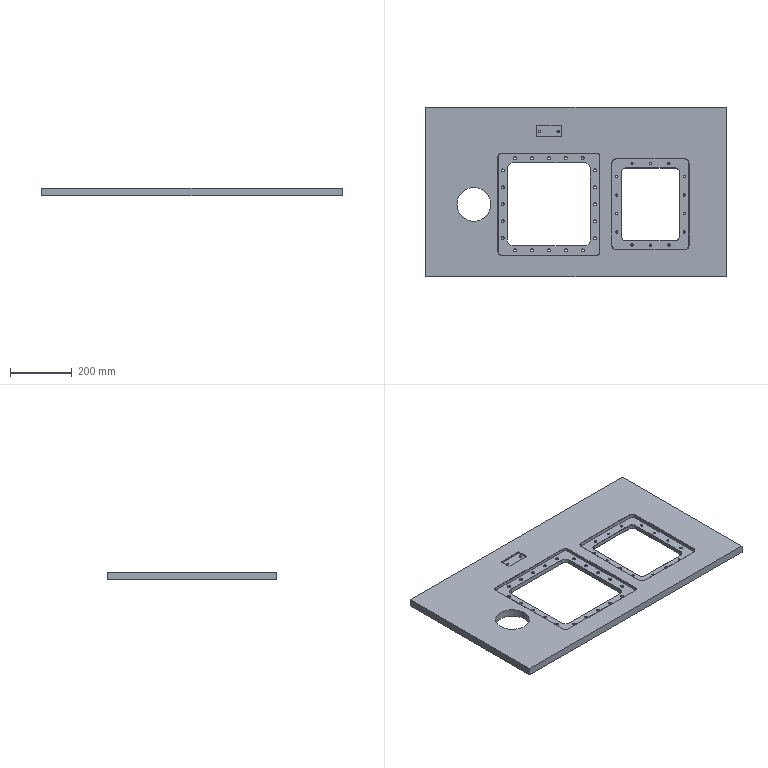Part | SolidWorks | features BaseBody 1 | 1 solid | 259 faces | box 976 x 550 x 25 mm | volume 9505923 mm3 | cone 120 | cylinder 90 | plane 49 | commonest cylinder face diameters 8.5 x40 6.5 x32 30 x8 20 x4 40 x4 110 x2